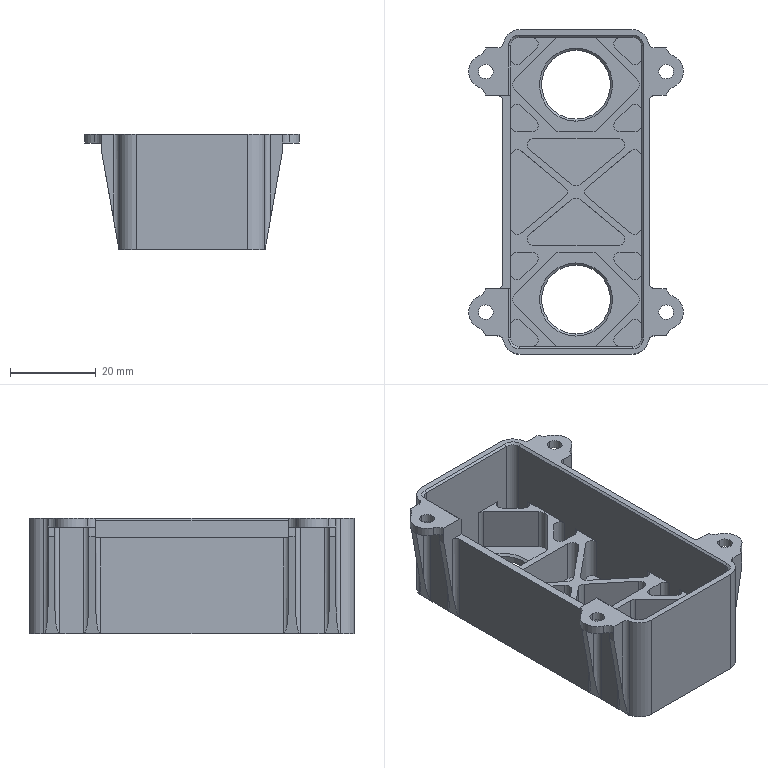NC program | NX | posted with a generic post | part box 50 x 75.58 x 26.8 mm
Lines 1 to 70 of 35818:
N10 G17 G21 G94 G90
(FLOOR_WALL_COPY_COPY , TOOL : D80)
N12 T19 M6
N14 G54
N16 G17 G0 G90 X0. Y82.79 S6500 M3
N18 G43 Z30. H19
N20 Z5.625
N22 G94 G1 Z2.625 F1500.
N24 Y77.79
N26 Y-77.79
N28 Y-82.79
N30 Z5.625
N32 G0 Z30.
N34 Y82.79
N36 Z4.75
N38 G1 Z1.75
N40 Y77.79
N42 Y-77.79
N44 Y-82.79
N46 Z4.75
N48 G0 Z30.
N50 Y82.79
N52 Z3.875
N54 G1 Z0.875
N56 Y77.79
N58 Y-77.79
N60 Y-82.79
N62 Z3.875
N64 G0 Z30.
N66 Y82.79
N68 Z3.
N70 G1 Z0.
N72 Y77.79
N74 Y-77.79
N76 Y-82.79
N78 Z3.
N80 G0 Z30.
N82 M5
(DRILLING_COPY_1 , TOOL : D6A45)
N84 T01 M6
N86 G54
N88 G17 G0 G90 X21. Y28. S5000 M3
N90 G43 Z30. H1
N92 G94 G81 G98 Z-1.1 F350. R3.
N94 X-21. Y-28.
N96 Y28.
N98 X21. Y-28.
N100 G80
N102 G0 X21. Y-28. Z30.
N104 M5
(DRILLING_COPY_1_COPY_1_1_COPY_1 , TOOL : 3.4ZT)
N106 T03 M6
N108 G54
N110 G17 G0 G90 X21. Y28. S2000 M3
N112 G43 Z30. H3
N114 G94 G83 G98 Z-4.521 F200. Q2. R3.
N116 X-21.
N118 Y-28.
N120 X21.
N122 G80
N124 G0 X21. Y-28. Z30.
N126 M5